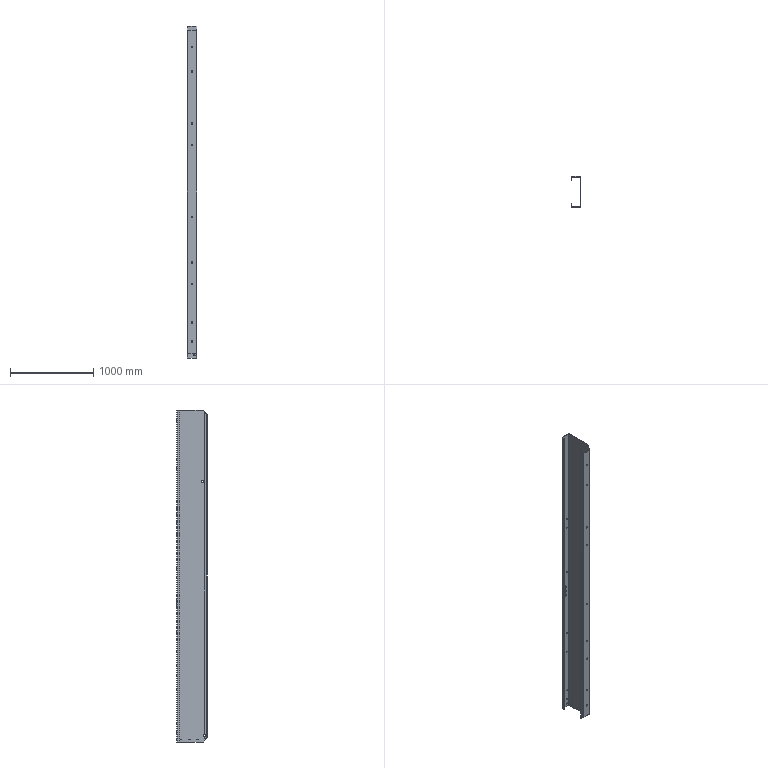Part | STEP file | VD-SYL0392DJ1006_1_1-1_VD-SYL03 | 1 solid | 190 faces | box 120 x 370 x 4000 mm | volume 15499432 mm3 | cylinder 98 | plane 84 | cone 6 | spline 2 | commonest cylinder face diameters 10 x42 18 x27 10.5 x12 28 x7 22 x4 6.917 x2